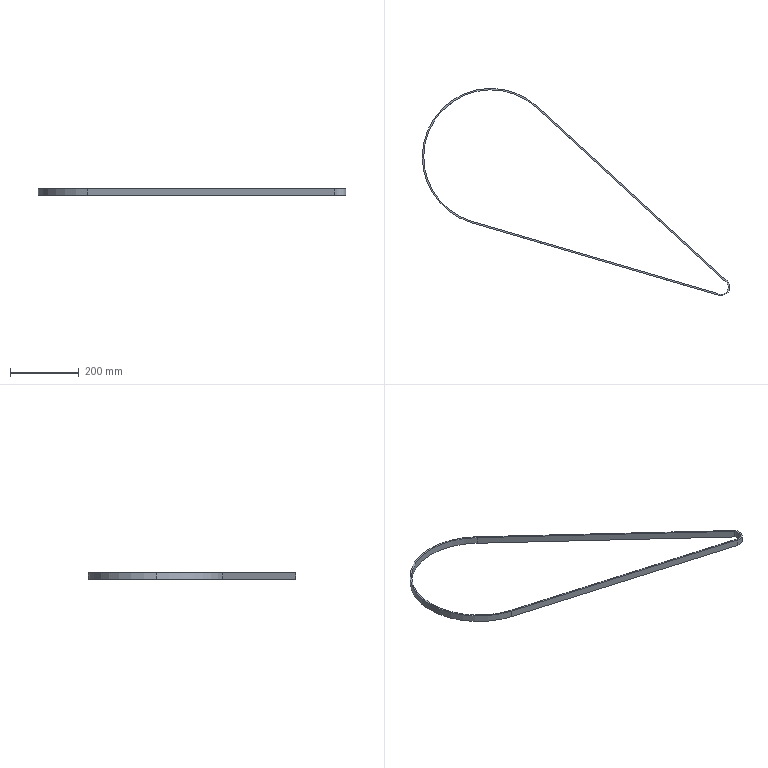Part | SolidWorks | features Sweep 1 | 1 solid | 12 faces | box 896.88 x 604.508 x 20 mm | volume 200125 mm3 | cylinder 6 | plane 6 | commonest cylinder face diameters 391.246 x2 400 x2 41.955 x1 50 x1
STEP:
#1=CARTESIAN_POINT('',(-652.123,298.999,10.));
#2=VERTEX_POINT('',#1);
#3=CARTESIAN_POINT('',(-795.816,490.91,10.));
#4=VERTEX_POINT('',#3);
#5=CARTESIAN_POINT('',(-595.816,490.91,10.));
#6=DIRECTION('',(0.,0.,-1.));
#7=DIRECTION('',(-1.,0.,0.));
#8=AXIS2_PLACEMENT_3D('',#5,#6,#7);
#9=CIRCLE('',#8,200.);
#10=EDGE_CURVE('',#2,#4,#9,.T.);
#11=ORIENTED_EDGE('',*,*,#10,.T.);
#12=CARTESIAN_POINT('',(-795.816,490.91,-10.));
#13=VERTEX_POINT('',#12);
#14=CARTESIAN_POINT('',(-795.816,490.91,0.));
#15=DIRECTION('',(0.,0.,-1.));
#16=VECTOR('',#15,1000.);
#17=LINE('',#14,#16);
#18=EDGE_CURVE('',#4,#13,#17,.T.);
#19=ORIENTED_EDGE('',*,*,#18,.T.);
#20=CARTESIAN_POINT('',(-652.123,298.999,-10.));
#21=VERTEX_POINT('',#20);
#22=CARTESIAN_POINT('',(-595.816,490.91,-10.));
#23=DIRECTION('',(0.,0.,-1.));
#24=DIRECTION('',(-1.,0.,0.));
#25=AXIS2_PLACEMENT_3D('',#22,#23,#24);
#26=CIRCLE('',#25,200.);
#27=EDGE_CURVE('',#21,#13,#26,.T.);
#28=ORIENTED_EDGE('',*,*,#27,.F.);
#29=CARTESIAN_POINT('',(-652.123,298.999,10.));
#30=DIRECTION('',(0.,0.,1.));
#31=VECTOR('',#30,1000.);
#32=LINE('',#29,#31);
#33=EDGE_CURVE('',#21,#2,#32,.T.);
#34=ORIENTED_EDGE('',*,*,#33,.T.);
#35=EDGE_LOOP('',(#11,#19,#28,#34));
#36=FACE_OUTER_BOUND('',#35,.T.);
#37=CARTESIAN_POINT('',(-595.816,490.91,0.));
#38=DIRECTION('',(0.,0.,-1.));
#39=DIRECTION('',(-1.,0.,0.));
#40=AXIS2_PLACEMENT_3D('',#37,#38,#39);
#41=CYLINDRICAL_SURFACE('',#40,200.);
#42=ADVANCED_FACE('',(#36),#41,.T.);
#43=CARTESIAN_POINT('',(-791.439,490.91,10.));
#44=VERTEX_POINT('',#43);
#45=CARTESIAN_POINT('',(-460.524,632.206,10.));
#46=VERTEX_POINT('',#45);
#47=CARTESIAN_POINT('',(-595.816,490.91,10.));
#48=DIRECTION('',(0.,0.,-1.));
#49=DIRECTION('',(-1.,0.,0.));
#50=AXIS2_PLACEMENT_3D('',#47,#48,#49);
#51=CIRCLE('',#50,195.623);
#52=EDGE_CURVE('',#44,#46,#51,.T.);
#53=ORIENTED_EDGE('',*,*,#52,.F.);
#54=CARTESIAN_POINT('',(-791.439,490.91,-10.));
#55=VERTEX_POINT('',#54);
#56=CARTESIAN_POINT('',(-791.439,490.91,0.));
#57=DIRECTION('',(0.,0.,-1.));
#58=VECTOR('',#57,1000.);
#59=LINE('',#56,#58);
#60=EDGE_CURVE('',#44,#55,#59,.T.);
#61=ORIENTED_EDGE('',*,*,#60,.T.);
#62=CARTESIAN_POINT('',(-460.524,632.206,-10.));
#63=VERTEX_POINT('',#62);
#64=CARTESIAN_POINT('',(-595.816,490.91,-10.));
#65=DIRECTION('',(0.,0.,-1.));
#66=DIRECTION('',(-1.,0.,0.));
#67=AXIS2_PLACEMENT_3D('',#64,#65,#66);
#68=CIRCLE('',#67,195.623);
#69=EDGE_CURVE('',#55,#63,#68,.T.);
#70=ORIENTED_EDGE('',*,*,#69,.T.);
#71=CARTESIAN_POINT('',(-460.524,632.206,10.));
#72=CARTESIAN_POINT('',(-460.524,632.206,3.333));
#73=CARTESIAN_POINT('',(-460.524,632.206,-3.333));
#74=CARTESIAN_POINT('',(-460.524,632.206,-10.));
#75=B_SPLINE_CURVE_WITH_KNOTS('',3,(#71,#72,#73,#74),.UNSPECIFIED.,.F.,.F.,(4,4),(0.,1.),.UNSPECIFIED.);
#76=EDGE_CURVE('',#46,#63,#75,.T.);
#77=ORIENTED_EDGE('',*,*,#76,.F.);
#78=EDGE_LOOP('',(#53,#61,#70,#77));
#79=FACE_OUTER_BOUND('',#78,.T.);
#80=CARTESIAN_POINT('',(-595.816,490.91,0.));
#81=DIRECTION('',(0.,0.,-1.));
#82=DIRECTION('',(-1.,0.,0.));
#83=AXIS2_PLACEMENT_3D('',#80,#81,#82);
#84=CYLINDRICAL_SURFACE('',#83,195.623);
#85=ADVANCED_FACE('',(#79),#84,.F.);
#86=ORIENTED_EDGE('',*,*,#60,.F.);
#87=CARTESIAN_POINT('',(-654.773,304.382,10.));
#88=VERTEX_POINT('',#87);
#89=CARTESIAN_POINT('',(-595.816,490.91,10.));
#90=DIRECTION('',(0.,0.,-1.));
#91=DIRECTION('',(-1.,0.,0.));
#92=AXIS2_PLACEMENT_3D('',#89,#90,#91);
#93=CIRCLE('',#92,195.623);
#94=EDGE_CURVE('',#88,#44,#93,.T.);
#95=ORIENTED_EDGE('',*,*,#94,.F.);
#96=CARTESIAN_POINT('',(-654.773,304.382,-10.));
#97=VERTEX_POINT('',#96);
#98=CARTESIAN_POINT('',(-654.773,304.382,10.));
#99=DIRECTION('',(0.,0.,-1.));
#100=VECTOR('',#99,1000.);
#101=LINE('',#98,#100);
#102=EDGE_CURVE('',#88,#97,#101,.T.);
#103=ORIENTED_EDGE('',*,*,#102,.T.);
#104=CARTESIAN_POINT('',(-595.816,490.91,-10.));
#105=DIRECTION('',(0.,0.,-1.));
#106=DIRECTION('',(-1.,0.,0.));
#107=AXIS2_PLACEMENT_3D('',#104,#105,#106);
#108=CIRCLE('',#107,195.623);
#109=EDGE_CURVE('',#97,#55,#108,.T.);
#110=ORIENTED_EDGE('',*,*,#109,.T.);
#111=EDGE_LOOP('',(#86,#95,#103,#110));
#112=FACE_OUTER_BOUND('',#111,.T.);
#113=CARTESIAN_POINT('',(-595.816,490.91,0.));
#114=DIRECTION('',(0.,0.,-1.));
#115=DIRECTION('',(-1.,0.,0.));
#116=AXIS2_PLACEMENT_3D('',#113,#114,#115);
#117=CYLINDRICAL_SURFACE('',#116,195.623);
#118=ADVANCED_FACE('',(#112),#117,.F.);
#119=ORIENTED_EDGE('',*,*,#18,.F.);
#120=CARTESIAN_POINT('',(-460.524,638.206,10.));
#121=VERTEX_POINT('',#120);
#122=CARTESIAN_POINT('',(-595.816,490.91,10.));
#123=DIRECTION('',(0.,0.,-1.));
#124=DIRECTION('',(-1.,0.,0.));
#125=AXIS2_PLACEMENT_3D('',#122,#123,#124);
#126=CIRCLE('',#125,200.);
#127=EDGE_CURVE('',#4,#121,#126,.T.);
#128=ORIENTED_EDGE('',*,*,#127,.T.);
#129=CARTESIAN_POINT('',(-460.524,638.206,-10.));
#130=VERTEX_POINT('',#129);
#131=CARTESIAN_POINT('',(-460.524,638.206,-10.));
#132=CARTESIAN_POINT('',(-460.524,638.206,-3.333));
#133=CARTESIAN_POINT('',(-460.524,638.206,3.333));
#134=CARTESIAN_POINT('',(-460.524,638.206,10.));
#135=B_SPLINE_CURVE_WITH_KNOTS('',3,(#131,#132,#133,#134),.UNSPECIFIED.,.F.,.F.,(4,4),(0.,1.),.UNSPECIFIED.);
#136=EDGE_CURVE('',#130,#121,#135,.T.);
#137=ORIENTED_EDGE('',*,*,#136,.F.);
#138=CARTESIAN_POINT('',(-595.816,490.91,-10.));
#139=DIRECTION('',(0.,0.,-1.));
#140=DIRECTION('',(-1.,0.,0.));
#141=AXIS2_PLACEMENT_3D('',#138,#139,#140);
#142=CIRCLE('',#141,200.);
#143=EDGE_CURVE('',#13,#130,#142,.T.);
#144=ORIENTED_EDGE('',*,*,#143,.F.);
#145=EDGE_LOOP('',(#119,#128,#137,#144));
#146=FACE_OUTER_BOUND('',#145,.T.);
#147=CARTESIAN_POINT('',(-595.816,490.91,0.));
#148=DIRECTION('',(0.,0.,-1.));
#149=DIRECTION('',(-1.,0.,0.));
#150=AXIS2_PLACEMENT_3D('',#147,#148,#149);
#151=CYLINDRICAL_SURFACE('',#150,200.);
#152=ADVANCED_FACE('',(#146),#151,.T.);
#153=CARTESIAN_POINT('',(66.376,92.795,10.));
#154=VERTEX_POINT('',#153);
#155=CARTESIAN_POINT('',(66.376,92.795,-10.));
#156=VERTEX_POINT('',#155);
#157=CARTESIAN_POINT('',(66.376,92.795,10.));
#158=DIRECTION('',(0.,0.,-1.));
#159=VECTOR('',#158,1000.);
#160=LINE('',#157,#159);
#161=EDGE_CURVE('',#154,#156,#160,.T.);
#162=ORIENTED_EDGE('',*,*,#161,.T.);
#163=CARTESIAN_POINT('',(66.376,92.795,-10.));
#164=DIRECTION('',(-0.9596,0.2815,0.));
#165=VECTOR('',#164,1000.);
#166=LINE('',#163,#165);
#167=EDGE_CURVE('',#156,#97,#166,.T.);
#168=ORIENTED_EDGE('',*,*,#167,.T.);
#169=ORIENTED_EDGE('',*,*,#102,.F.);
#170=CARTESIAN_POINT('',(66.376,92.795,10.));
#171=DIRECTION('',(-0.9596,0.2815,0.));
#172=VECTOR('',#171,1000.);
#173=LINE('',#170,#172);
#174=EDGE_CURVE('',#154,#88,#173,.T.);
#175=ORIENTED_EDGE('',*,*,#174,.F.);
#176=EDGE_LOOP('',(#162,#168,#169,#175));
#177=FACE_OUTER_BOUND('',#176,.T.);
#178=CARTESIAN_POINT('',(66.376,92.795,10.));
#179=DIRECTION('',(0.2815,0.9596,0.));
#180=DIRECTION('',(-0.9596,0.2815,0.));
#181=AXIS2_PLACEMENT_3D('',#178,#179,#180);
#182=PLANE('',#181);
#183=ADVANCED_FACE('',(#177),#182,.T.);
#184=CARTESIAN_POINT('',(69.026,87.413,-10.));
#185=VERTEX_POINT('',#184);
#186=CARTESIAN_POINT('',(69.026,87.413,10.));
#187=VERTEX_POINT('',#186);
#188=CARTESIAN_POINT('',(69.026,87.413,10.));
#189=DIRECTION('',(0.,0.,1.));
#190=VECTOR('',#189,1000.);
#191=LINE('',#188,#190);
#192=EDGE_CURVE('',#185,#187,#191,.T.);
#193=ORIENTED_EDGE('',*,*,#192,.T.);
#194=CARTESIAN_POINT('',(69.026,87.413,10.));
#195=DIRECTION('',(-0.9596,0.2815,0.));
#196=VECTOR('',#195,1000.);
#197=LINE('',#194,#196);
#198=EDGE_CURVE('',#187,#2,#197,.T.);
#199=ORIENTED_EDGE('',*,*,#198,.T.);
#200=ORIENTED_EDGE('',*,*,#33,.F.);
#201=CARTESIAN_POINT('',(69.026,87.413,-10.));
#202=DIRECTION('',(-0.9596,0.2815,0.));
#203=VECTOR('',#202,1000.);
#204=LINE('',#201,#203);
#205=EDGE_CURVE('',#185,#21,#204,.T.);
#206=ORIENTED_EDGE('',*,*,#205,.F.);
#207=EDGE_LOOP('',(#193,#199,#200,#206));
#208=FACE_OUTER_BOUND('',#207,.T.);
#209=CARTESIAN_POINT('',(69.026,87.413,10.));
#210=DIRECTION('',(-0.2815,-0.9596,0.));
#211=DIRECTION('',(0.9596,-0.2815,0.));
#212=AXIS2_PLACEMENT_3D('',#209,#210,#211);
#213=PLANE('',#212);
#214=ADVANCED_FACE('',(#208),#213,.T.);
#215=CARTESIAN_POINT('',(92.976,123.813,10.));
#216=VERTEX_POINT('',#215);
#217=CARTESIAN_POINT('',(92.976,123.813,-10.));
#218=VERTEX_POINT('',#217);
#219=CARTESIAN_POINT('',(92.976,123.813,10.));
#220=DIRECTION('',(0.,0.,-1.));
#221=VECTOR('',#220,1000.);
#222=LINE('',#219,#221);
#223=EDGE_CURVE('',#216,#218,#222,.T.);
#224=ORIENTED_EDGE('',*,*,#223,.T.);
#225=CARTESIAN_POINT('',(76.064,111.401,-10.));
#226=DIRECTION('',(0.,0.,-1.));
#227=DIRECTION('',(-1.,0.,0.));
#228=AXIS2_PLACEMENT_3D('',#225,#226,#227);
#229=CIRCLE('',#228,20.978);
#230=EDGE_CURVE('',#218,#156,#229,.T.);
#231=ORIENTED_EDGE('',*,*,#230,.T.);
#232=ORIENTED_EDGE('',*,*,#161,.F.);
#233=CARTESIAN_POINT('',(76.064,111.401,10.));
#234=DIRECTION('',(0.,0.,-1.));
#235=DIRECTION('',(-1.,0.,0.));
#236=AXIS2_PLACEMENT_3D('',#233,#234,#235);
#237=CIRCLE('',#236,20.978);
#238=EDGE_CURVE('',#216,#154,#237,.T.);
#239=ORIENTED_EDGE('',*,*,#238,.F.);
#240=EDGE_LOOP('',(#224,#231,#232,#239));
#241=FACE_OUTER_BOUND('',#240,.T.);
#242=CARTESIAN_POINT('',(76.064,111.401,0.));
#243=DIRECTION('',(0.,0.,-1.));
#244=DIRECTION('',(-1.,0.,0.));
#245=AXIS2_PLACEMENT_3D('',#242,#243,#244);
#246=CYLINDRICAL_SURFACE('',#245,20.978);
#247=ADVANCED_FACE('',(#241),#246,.F.);
#248=CARTESIAN_POINT('',(92.976,129.813,-10.));
#249=VERTEX_POINT('',#248);
#250=CARTESIAN_POINT('',(92.976,129.813,10.));
#251=VERTEX_POINT('',#250);
#252=CARTESIAN_POINT('',(92.976,129.813,10.));
#253=DIRECTION('',(0.,0.,1.));
#254=VECTOR('',#253,1000.);
#255=LINE('',#252,#254);
#256=EDGE_CURVE('',#249,#251,#255,.T.);
#257=ORIENTED_EDGE('',*,*,#256,.T.);
#258=CARTESIAN_POINT('',(76.064,111.401,10.));
#259=DIRECTION('',(0.,0.,-1.));
#260=DIRECTION('',(-1.,0.,0.));
#261=AXIS2_PLACEMENT_3D('',#258,#259,#260);
#262=CIRCLE('',#261,25.);
#263=EDGE_CURVE('',#251,#187,#262,.T.);
#264=ORIENTED_EDGE('',*,*,#263,.T.);
#265=ORIENTED_EDGE('',*,*,#192,.F.);
#266=CARTESIAN_POINT('',(76.064,111.401,-10.));
#267=DIRECTION('',(0.,0.,-1.));
#268=DIRECTION('',(-1.,0.,0.));
#269=AXIS2_PLACEMENT_3D('',#266,#267,#268);
#270=CIRCLE('',#269,25.);
#271=EDGE_CURVE('',#249,#185,#270,.T.);
#272=ORIENTED_EDGE('',*,*,#271,.F.);
#273=EDGE_LOOP('',(#257,#264,#265,#272));
#274=FACE_OUTER_BOUND('',#273,.T.);
#275=CARTESIAN_POINT('',(76.064,111.401,0.));
#276=DIRECTION('',(0.,0.,-1.));
#277=DIRECTION('',(-1.,0.,0.));
#278=AXIS2_PLACEMENT_3D('',#275,#276,#277);
#279=CYLINDRICAL_SURFACE('',#278,25.);
#280=ADVANCED_FACE('',(#274),#279,.T.);
#281=CARTESIAN_POINT('',(92.976,123.813,10.));
#282=DIRECTION('',(-0.7365,0.6765,0.));
#283=VECTOR('',#282,1000.);
#284=LINE('',#281,#283);
#285=EDGE_CURVE('',#216,#46,#284,.T.);
#286=ORIENTED_EDGE('',*,*,#285,.F.);
#287=ORIENTED_EDGE('',*,*,#238,.T.);
#288=ORIENTED_EDGE('',*,*,#174,.T.);
#289=ORIENTED_EDGE('',*,*,#94,.T.);
#290=ORIENTED_EDGE('',*,*,#52,.T.);
#291=EDGE_LOOP('',(#286,#287,#288,#289,#290));
#292=FACE_BOUND('',#291,.T.);
#293=CARTESIAN_POINT('',(92.976,129.813,10.));
#294=DIRECTION('',(-0.7365,0.6765,0.));
#295=VECTOR('',#294,1000.);
#296=LINE('',#293,#295);
#297=EDGE_CURVE('',#251,#121,#296,.T.);
#298=ORIENTED_EDGE('',*,*,#297,.T.);
#299=ORIENTED_EDGE('',*,*,#127,.F.);
#300=ORIENTED_EDGE('',*,*,#10,.F.);
#301=ORIENTED_EDGE('',*,*,#198,.F.);
#302=ORIENTED_EDGE('',*,*,#263,.F.);
#303=EDGE_LOOP('',(#298,#299,#300,#301,#302));
#304=FACE_OUTER_BOUND('',#303,.T.);
#305=CARTESIAN_POINT('',(92.976,129.813,10.));
#306=DIRECTION('',(0.,0.,-1.));
#307=DIRECTION('',(-1.,0.,0.));
#308=AXIS2_PLACEMENT_3D('',#305,#306,#307);
#309=PLANE('',#308);
#310=ADVANCED_FACE('',(#292,#304),#309,.F.);
#311=ORIENTED_EDGE('',*,*,#76,.T.);
#312=CARTESIAN_POINT('',(92.976,123.813,-10.));
#313=DIRECTION('',(-0.7365,0.6765,0.));
#314=VECTOR('',#313,1000.);
#315=LINE('',#312,#314);
#316=EDGE_CURVE('',#218,#63,#315,.T.);
#317=ORIENTED_EDGE('',*,*,#316,.F.);
#318=ORIENTED_EDGE('',*,*,#223,.F.);
#319=ORIENTED_EDGE('',*,*,#285,.T.);
#320=EDGE_LOOP('',(#311,#317,#318,#319));
#321=FACE_OUTER_BOUND('',#320,.T.);
#322=CARTESIAN_POINT('',(92.976,123.813,10.));
#323=DIRECTION('',(0.6765,0.7365,0.));
#324=DIRECTION('',(-0.7365,0.6765,0.));
#325=AXIS2_PLACEMENT_3D('',#322,#323,#324);
#326=PLANE('',#325);
#327=ADVANCED_FACE('',(#321),#326,.F.);
#328=CARTESIAN_POINT('',(92.976,129.813,-10.));
#329=DIRECTION('',(-0.7365,0.6765,0.));
#330=VECTOR('',#329,1000.);
#331=LINE('',#328,#330);
#332=EDGE_CURVE('',#249,#130,#331,.T.);
#333=ORIENTED_EDGE('',*,*,#332,.F.);
#334=ORIENTED_EDGE('',*,*,#271,.T.);
#335=ORIENTED_EDGE('',*,*,#205,.T.);
#336=ORIENTED_EDGE('',*,*,#27,.T.);
#337=ORIENTED_EDGE('',*,*,#143,.T.);
#338=EDGE_LOOP('',(#333,#334,#335,#336,#337));
#339=FACE_OUTER_BOUND('',#338,.T.);
#340=ORIENTED_EDGE('',*,*,#316,.T.);
#341=ORIENTED_EDGE('',*,*,#69,.F.);
#342=ORIENTED_EDGE('',*,*,#109,.F.);
#343=ORIENTED_EDGE('',*,*,#167,.F.);
#344=ORIENTED_EDGE('',*,*,#230,.F.);
#345=EDGE_LOOP('',(#340,#341,#342,#343,#344));
#346=FACE_BOUND('',#345,.T.);
#347=CARTESIAN_POINT('',(92.976,129.813,-10.));
#348=DIRECTION('',(0.,0.,1.));
#349=DIRECTION('',(1.,0.,0.));
#350=AXIS2_PLACEMENT_3D('',#347,#348,#349);
#351=PLANE('',#350);
#352=ADVANCED_FACE('',(#339,#346),#351,.F.);
#353=ORIENTED_EDGE('',*,*,#136,.T.);
#354=ORIENTED_EDGE('',*,*,#297,.F.);
#355=ORIENTED_EDGE('',*,*,#256,.F.);
#356=ORIENTED_EDGE('',*,*,#332,.T.);
#357=EDGE_LOOP('',(#353,#354,#355,#356));
#358=FACE_OUTER_BOUND('',#357,.T.);
#359=CARTESIAN_POINT('',(92.976,129.813,10.));
#360=DIRECTION('',(-0.6765,-0.7365,0.));
#361=DIRECTION('',(0.7365,-0.6765,0.));
#362=AXIS2_PLACEMENT_3D('',#359,#360,#361);
#363=PLANE('',#362);
#364=ADVANCED_FACE('',(#358),#363,.F.);
#365=CLOSED_SHELL('',(#42,#85,#118,#152,#183,#214,#247,#280,#310,#327,#352,#364));
#366=MANIFOLD_SOLID_BREP('',#365);
#367=CARTESIAN_POINT('',(0.,0.,0.));
#368=DIRECTION('',(0.,0.,1.));
#369=DIRECTION('',(1.,0.,0.));
#370=AXIS2_PLACEMENT_3D('',#367,#368,#369);
#371=(LENGTH_UNIT()NAMED_UNIT(*)SI_UNIT(.MILLI.,.METRE.));
#372=UNCERTAINTY_MEASURE_WITH_UNIT(LENGTH_MEASURE(0.00001),#371,'','');
#373=(NAMED_UNIT(*)PLANE_ANGLE_UNIT()SI_UNIT($,.RADIAN.));
#374=(NAMED_UNIT(*)SI_UNIT($,.STERADIAN.)SOLID_ANGLE_UNIT());
#375=(GEOMETRIC_REPRESENTATION_CONTEXT(3)GLOBAL_UNCERTAINTY_ASSIGNED_CONTEXT((#372))GLOBAL_UNIT_ASSIGNED_CONTEXT((#371,#373,#374))REPRESENTATION_CONTEXT('',''));
#376=ADVANCED_BREP_SHAPE_REPRESENTATION('',(#366,#370),#375);